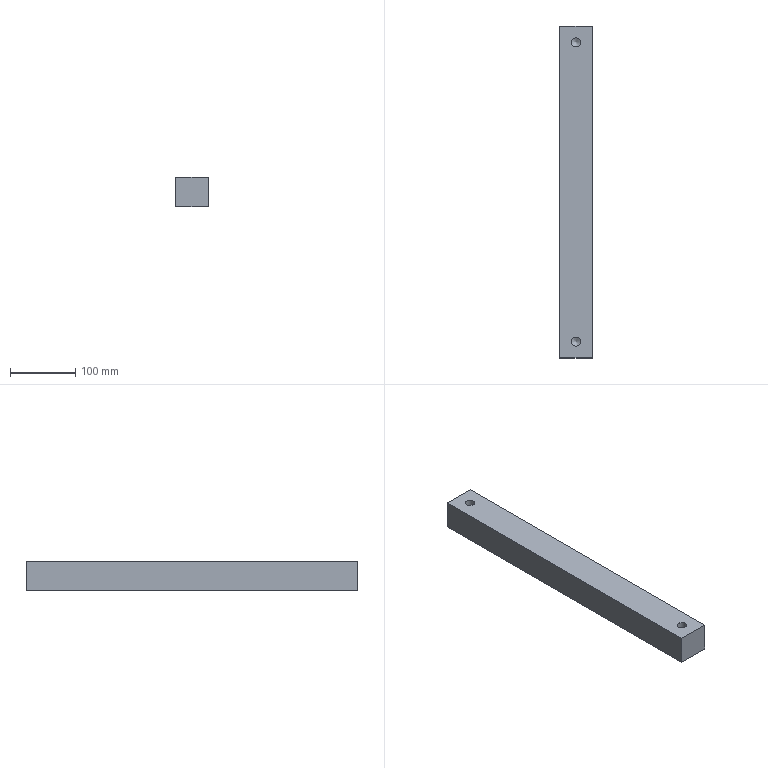Part | STEP file | 023_id2182_x_t | 1 solid | 10 faces | box 50 x 510 x 45 mm | volume 1141094 mm3 | plane 6 | cylinder 2 | cone 2 | commonest cylinder face diameters 14 x2
STEP:
#1=CARTESIAN_POINT('',(0.,0.,0.));
#2=DIRECTION('',(0.,0.,1.));
#3=DIRECTION('',(1.,0.,0.));
#4=AXIS2_PLACEMENT_3D('',#1,#2,#3);
#5=CARTESIAN_POINT('',(716.5,230.,230.));
#6=VERTEX_POINT('',#5);
#7=CARTESIAN_POINT('',(730.5,230.,230.));
#8=VERTEX_POINT('',#7);
#9=CARTESIAN_POINT('',(723.5,230.,230.));
#10=DIRECTION('',(0.,0.,1.));
#11=DIRECTION('',(-1.,0.,0.));
#12=AXIS2_PLACEMENT_3D('',#9,#10,#11);
#13=CIRCLE('',#12,7.);
#14=CARTESIAN_POINT('',(903.5,-140.,230.));
#15=DIRECTION('',(0.,0.,1.));
#16=DIRECTION('',(1.,0.,0.));
#17=AXIS2_PLACEMENT_3D('',#14,#15,#16);
#18=PLANE('',#17);
#19=CARTESIAN_POINT('',(-180.,370.));
#20=DIRECTION('',(-1.,0.));
#21=AXIS2_PLACEMENT_2D('',#19,#20);
#22=CIRCLE('',#21,7.);
#23=(GEOMETRIC_REPRESENTATION_CONTEXT(2)PARAMETRIC_REPRESENTATION_CONTEXT()REPRESENTATION_CONTEXT('',''));
#24=DEFINITIONAL_REPRESENTATION('',(#22),#23);
#25=PCURVE('',#18,#24);
#26=CARTESIAN_POINT('',(723.5,230.,279.));
#27=DIRECTION('',(0.,0.,-1.));
#28=DIRECTION('',(1.,0.,0.));
#29=AXIS2_PLACEMENT_3D('',#26,#27,#28);
#30=CYLINDRICAL_SURFACE('',#29,7.);
#31=CARTESIAN_POINT('',(3.142,49.));
#32=DIRECTION('',(-1.,0.));
#33=VECTOR('',#32,1.);
#34=LINE('',#31,#33);
#35=(GEOMETRIC_REPRESENTATION_CONTEXT(2)PARAMETRIC_REPRESENTATION_CONTEXT()REPRESENTATION_CONTEXT('',''));
#36=DEFINITIONAL_REPRESENTATION('',(#34),#35);
#37=PCURVE('',#30,#36);
#38=SURFACE_CURVE('',#13,(#25,#37),.PCURVE_S1.);
#39=EDGE_CURVE('',#6,#8,#38,.T.);
#40=ORIENTED_EDGE('',*,*,#39,.F.);
#41=CARTESIAN_POINT('',(723.5,230.,230.));
#42=DIRECTION('',(0.,0.,1.));
#43=DIRECTION('',(-1.,0.,0.));
#44=AXIS2_PLACEMENT_3D('',#41,#42,#43);
#45=CIRCLE('',#44,7.);
#46=CARTESIAN_POINT('',(-180.,370.));
#47=DIRECTION('',(-1.,0.));
#48=AXIS2_PLACEMENT_2D('',#46,#47);
#49=CIRCLE('',#48,7.);
#50=(GEOMETRIC_REPRESENTATION_CONTEXT(2)PARAMETRIC_REPRESENTATION_CONTEXT()REPRESENTATION_CONTEXT('',''));
#51=DEFINITIONAL_REPRESENTATION('',(#49),#50);
#52=PCURVE('',#18,#51);
#53=CARTESIAN_POINT('',(9.425,49.));
#54=DIRECTION('',(-1.,0.));
#55=VECTOR('',#54,1.);
#56=LINE('',#53,#55);
#57=(GEOMETRIC_REPRESENTATION_CONTEXT(2)PARAMETRIC_REPRESENTATION_CONTEXT()REPRESENTATION_CONTEXT('',''));
#58=DEFINITIONAL_REPRESENTATION('',(#56),#57);
#59=PCURVE('',#30,#58);
#60=SURFACE_CURVE('',#45,(#52,#59),.PCURVE_S1.);
#61=EDGE_CURVE('',#8,#6,#60,.T.);
#62=ORIENTED_EDGE('',*,*,#61,.F.);
#63=EDGE_LOOP('',(#40,#62));
#64=FACE_BOUND('',#63,.T.);
#65=CARTESIAN_POINT('',(716.5,-230.,230.));
#66=VERTEX_POINT('',#65);
#67=CARTESIAN_POINT('',(730.5,-230.,230.));
#68=VERTEX_POINT('',#67);
#69=CARTESIAN_POINT('',(723.5,-230.,230.));
#70=DIRECTION('',(0.,0.,-1.));
#71=DIRECTION('',(-1.,0.,0.));
#72=AXIS2_PLACEMENT_3D('',#69,#70,#71);
#73=CIRCLE('',#72,7.);
#74=CARTESIAN_POINT('',(-187.,-90.));
#75=CARTESIAN_POINT('',(-187.,-77.876));
#76=CARTESIAN_POINT('',(-176.5,-83.938));
#77=CARTESIAN_POINT('',(-166.,-90.));
#78=CARTESIAN_POINT('',(-176.5,-96.062));
#79=CARTESIAN_POINT('',(-187.,-102.124));
#80=CARTESIAN_POINT('',(-187.,-90.));
#81=(BOUNDED_CURVE()B_SPLINE_CURVE(2,(#74,#75,#76,#77,#78,#79,#80),.UNSPECIFIED.,.T.,.F.)B_SPLINE_CURVE_WITH_KNOTS((1,2,2,2,2,1),(-2.094,0.,2.094,4.189,6.283,8.378),.UNSPECIFIED.)CURVE()GEOMETRIC_REPRESENTATION_ITEM()RATIONAL_B_SPLINE_CURVE((1.,0.5,1.,0.5,1.,0.5,1.))REPRESENTATION_ITEM(''));
#82=(GEOMETRIC_REPRESENTATION_CONTEXT(2)PARAMETRIC_REPRESENTATION_CONTEXT()REPRESENTATION_CONTEXT('',''));
#83=DEFINITIONAL_REPRESENTATION('',(#81),#82);
#84=PCURVE('',#18,#83);
#85=CARTESIAN_POINT('',(723.5,-230.,279.));
#86=DIRECTION('',(0.,0.,-1.));
#87=DIRECTION('',(1.,0.,0.));
#88=AXIS2_PLACEMENT_3D('',#85,#86,#87);
#89=CYLINDRICAL_SURFACE('',#88,7.);
#90=CARTESIAN_POINT('',(3.142,49.));
#91=DIRECTION('',(1.,0.));
#92=VECTOR('',#91,1.);
#93=LINE('',#90,#92);
#94=(GEOMETRIC_REPRESENTATION_CONTEXT(2)PARAMETRIC_REPRESENTATION_CONTEXT()REPRESENTATION_CONTEXT('',''));
#95=DEFINITIONAL_REPRESENTATION('',(#93),#94);
#96=PCURVE('',#89,#95);
#97=SURFACE_CURVE('',#73,(#84,#96),.PCURVE_S1.);
#98=EDGE_CURVE('',#66,#68,#97,.T.);
#99=ORIENTED_EDGE('',*,*,#98,.T.);
#100=CARTESIAN_POINT('',(723.5,-230.,230.));
#101=DIRECTION('',(0.,0.,-1.));
#102=DIRECTION('',(-1.,0.,0.));
#103=AXIS2_PLACEMENT_3D('',#100,#101,#102);
#104=CIRCLE('',#103,7.);
#105=CARTESIAN_POINT('',(-187.,-90.));
#106=CARTESIAN_POINT('',(-187.,-77.876));
#107=CARTESIAN_POINT('',(-176.5,-83.938));
#108=CARTESIAN_POINT('',(-166.,-90.));
#109=CARTESIAN_POINT('',(-176.5,-96.062));
#110=CARTESIAN_POINT('',(-187.,-102.124));
#111=CARTESIAN_POINT('',(-187.,-90.));
#112=(BOUNDED_CURVE()B_SPLINE_CURVE(2,(#105,#106,#107,#108,#109,#110,#111),.UNSPECIFIED.,.T.,.F.)B_SPLINE_CURVE_WITH_KNOTS((1,2,2,2,2,1),(-2.094,0.,2.094,4.189,6.283,8.378),.UNSPECIFIED.)CURVE()GEOMETRIC_REPRESENTATION_ITEM()RATIONAL_B_SPLINE_CURVE((1.,0.5,1.,0.5,1.,0.5,1.))REPRESENTATION_ITEM(''));
#113=(GEOMETRIC_REPRESENTATION_CONTEXT(2)PARAMETRIC_REPRESENTATION_CONTEXT()REPRESENTATION_CONTEXT('',''));
#114=DEFINITIONAL_REPRESENTATION('',(#112),#113);
#115=PCURVE('',#18,#114);
#116=CARTESIAN_POINT('',(-3.142,49.));
#117=DIRECTION('',(1.,0.));
#118=VECTOR('',#117,1.);
#119=LINE('',#116,#118);
#120=(GEOMETRIC_REPRESENTATION_CONTEXT(2)PARAMETRIC_REPRESENTATION_CONTEXT()REPRESENTATION_CONTEXT('',''));
#121=DEFINITIONAL_REPRESENTATION('',(#119),#120);
#122=PCURVE('',#89,#121);
#123=SURFACE_CURVE('',#104,(#115,#122),.PCURVE_S1.);
#124=EDGE_CURVE('',#68,#66,#123,.T.);
#125=ORIENTED_EDGE('',*,*,#124,.T.);
#126=EDGE_LOOP('',(#99,#125));
#127=FACE_BOUND('',#126,.T.);
#128=CARTESIAN_POINT('',(748.5,255.,230.));
#129=VERTEX_POINT('',#128);
#130=CARTESIAN_POINT('',(698.5,255.,230.));
#131=VERTEX_POINT('',#130);
#132=CARTESIAN_POINT('',(698.5,255.,230.));
#133=DIRECTION('',(-1.,0.,0.));
#134=VECTOR('',#133,1.);
#135=LINE('',#132,#134);
#136=CARTESIAN_POINT('',(-205.,395.));
#137=DIRECTION('',(-1.,0.));
#138=VECTOR('',#137,1.);
#139=LINE('',#136,#138);
#140=(GEOMETRIC_REPRESENTATION_CONTEXT(2)PARAMETRIC_REPRESENTATION_CONTEXT()REPRESENTATION_CONTEXT('',''));
#141=DEFINITIONAL_REPRESENTATION('',(#139),#140);
#142=PCURVE('',#18,#141);
#143=CARTESIAN_POINT('',(698.5,255.,428.5));
#144=DIRECTION('',(0.,1.,0.));
#145=DIRECTION('',(0.,0.,1.));
#146=AXIS2_PLACEMENT_3D('',#143,#144,#145);
#147=PLANE('',#146);
#148=CARTESIAN_POINT('',(-198.5,0.));
#149=DIRECTION('',(0.,-1.));
#150=VECTOR('',#149,1.);
#151=LINE('',#148,#150);
#152=(GEOMETRIC_REPRESENTATION_CONTEXT(2)PARAMETRIC_REPRESENTATION_CONTEXT()REPRESENTATION_CONTEXT('',''));
#153=DEFINITIONAL_REPRESENTATION('',(#151),#152);
#154=PCURVE('',#147,#153);
#155=SURFACE_CURVE('',#135,(#142,#154),.PCURVE_S1.);
#156=EDGE_CURVE('',#129,#131,#155,.T.);
#157=ORIENTED_EDGE('',*,*,#156,.T.);
#158=CARTESIAN_POINT('',(698.5,-255.,230.));
#159=VERTEX_POINT('',#158);
#160=CARTESIAN_POINT('',(698.5,-350.,230.));
#161=DIRECTION('',(0.,-1.,0.));
#162=VECTOR('',#161,1.);
#163=LINE('',#160,#162);
#164=CARTESIAN_POINT('',(-205.,-210.));
#165=DIRECTION('',(0.,-1.));
#166=VECTOR('',#165,1.);
#167=LINE('',#164,#166);
#168=(GEOMETRIC_REPRESENTATION_CONTEXT(2)PARAMETRIC_REPRESENTATION_CONTEXT()REPRESENTATION_CONTEXT('',''));
#169=DEFINITIONAL_REPRESENTATION('',(#167),#168);
#170=PCURVE('',#18,#169);
#171=CARTESIAN_POINT('',(698.5,-350.,428.5));
#172=DIRECTION('',(-1.,0.,0.));
#173=DIRECTION('',(0.,0.,-1.));
#174=AXIS2_PLACEMENT_3D('',#171,#172,#173);
#175=PLANE('',#174);
#176=CARTESIAN_POINT('',(198.5,0.));
#177=DIRECTION('',(0.,1.));
#178=VECTOR('',#177,1.);
#179=LINE('',#176,#178);
#180=(GEOMETRIC_REPRESENTATION_CONTEXT(2)PARAMETRIC_REPRESENTATION_CONTEXT()REPRESENTATION_CONTEXT('',''));
#181=DEFINITIONAL_REPRESENTATION('',(#179),#180);
#182=PCURVE('',#175,#181);
#183=SURFACE_CURVE('',#163,(#170,#182),.PCURVE_S1.);
#184=EDGE_CURVE('',#131,#159,#183,.T.);
#185=ORIENTED_EDGE('',*,*,#184,.T.);
#186=CARTESIAN_POINT('',(748.5,-255.,230.));
#187=VERTEX_POINT('',#186);
#188=CARTESIAN_POINT('',(698.5,-255.,230.));
#189=DIRECTION('',(-1.,0.,0.));
#190=VECTOR('',#189,1.);
#191=LINE('',#188,#190);
#192=CARTESIAN_POINT('',(-205.,-115.));
#193=DIRECTION('',(-1.,0.));
#194=VECTOR('',#193,1.);
#195=LINE('',#192,#194);
#196=(GEOMETRIC_REPRESENTATION_CONTEXT(2)PARAMETRIC_REPRESENTATION_CONTEXT()REPRESENTATION_CONTEXT('',''));
#197=DEFINITIONAL_REPRESENTATION('',(#195),#196);
#198=PCURVE('',#18,#197);
#199=CARTESIAN_POINT('',(698.5,-255.,428.5));
#200=DIRECTION('',(0.,1.,0.));
#201=DIRECTION('',(0.,0.,1.));
#202=AXIS2_PLACEMENT_3D('',#199,#200,#201);
#203=PLANE('',#202);
#204=CARTESIAN_POINT('',(-198.5,0.));
#205=DIRECTION('',(0.,-1.));
#206=VECTOR('',#205,1.);
#207=LINE('',#204,#206);
#208=(GEOMETRIC_REPRESENTATION_CONTEXT(2)PARAMETRIC_REPRESENTATION_CONTEXT()REPRESENTATION_CONTEXT('',''));
#209=DEFINITIONAL_REPRESENTATION('',(#207),#208);
#210=PCURVE('',#203,#209);
#211=SURFACE_CURVE('',#191,(#198,#210),.PCURVE_S1.);
#212=EDGE_CURVE('',#187,#159,#211,.T.);
#213=ORIENTED_EDGE('',*,*,#212,.F.);
#214=CARTESIAN_POINT('',(748.5,-350.,230.));
#215=DIRECTION('',(0.,1.,0.));
#216=VECTOR('',#215,1.);
#217=LINE('',#214,#216);
#218=CARTESIAN_POINT('',(-155.,-210.));
#219=DIRECTION('',(0.,1.));
#220=VECTOR('',#219,1.);
#221=LINE('',#218,#220);
#222=(GEOMETRIC_REPRESENTATION_CONTEXT(2)PARAMETRIC_REPRESENTATION_CONTEXT()REPRESENTATION_CONTEXT('',''));
#223=DEFINITIONAL_REPRESENTATION('',(#221),#222);
#224=PCURVE('',#18,#223);
#225=CARTESIAN_POINT('',(748.5,-350.,428.5));
#226=DIRECTION('',(-1.,0.,0.));
#227=DIRECTION('',(0.,0.,-1.));
#228=AXIS2_PLACEMENT_3D('',#225,#226,#227);
#229=PLANE('',#228);
#230=CARTESIAN_POINT('',(198.5,0.));
#231=DIRECTION('',(0.,-1.));
#232=VECTOR('',#231,1.);
#233=LINE('',#230,#232);
#234=(GEOMETRIC_REPRESENTATION_CONTEXT(2)PARAMETRIC_REPRESENTATION_CONTEXT()REPRESENTATION_CONTEXT('',''));
#235=DEFINITIONAL_REPRESENTATION('',(#233),#234);
#236=PCURVE('',#229,#235);
#237=SURFACE_CURVE('',#217,(#224,#236),.PCURVE_S1.);
#238=EDGE_CURVE('',#187,#129,#237,.T.);
#239=ORIENTED_EDGE('',*,*,#238,.T.);
#240=EDGE_LOOP('',(#157,#185,#213,#239));
#241=FACE_BOUND('',#240,.T.);
#242=ADVANCED_FACE('',(#64,#127,#241),#18,.T.);
#243=CARTESIAN_POINT('',(748.5,-255.,185.));
#244=VERTEX_POINT('',#243);
#245=CARTESIAN_POINT('',(698.5,-255.,185.));
#246=VERTEX_POINT('',#245);
#247=CARTESIAN_POINT('',(698.5,-255.,185.));
#248=DIRECTION('',(-1.,0.,0.));
#249=VECTOR('',#248,1.);
#250=LINE('',#247,#249);
#251=CARTESIAN_POINT('',(698.5,-350.,185.));
#252=DIRECTION('',(0.,0.,1.));
#253=DIRECTION('',(0.,-1.,0.));
#254=AXIS2_PLACEMENT_3D('',#251,#252,#253);
#255=PLANE('',#254);
#256=CARTESIAN_POINT('',(-95.,0.));
#257=DIRECTION('',(0.,-1.));
#258=VECTOR('',#257,1.);
#259=LINE('',#256,#258);
#260=(GEOMETRIC_REPRESENTATION_CONTEXT(2)PARAMETRIC_REPRESENTATION_CONTEXT()REPRESENTATION_CONTEXT('',''));
#261=DEFINITIONAL_REPRESENTATION('',(#259),#260);
#262=PCURVE('',#255,#261);
#263=CARTESIAN_POINT('',(-243.5,0.));
#264=DIRECTION('',(0.,-1.));
#265=VECTOR('',#264,1.);
#266=LINE('',#263,#265);
#267=(GEOMETRIC_REPRESENTATION_CONTEXT(2)PARAMETRIC_REPRESENTATION_CONTEXT()REPRESENTATION_CONTEXT('',''));
#268=DEFINITIONAL_REPRESENTATION('',(#266),#267);
#269=PCURVE('',#203,#268);
#270=SURFACE_CURVE('',#250,(#262,#269),.PCURVE_S1.);
#271=EDGE_CURVE('',#244,#246,#270,.T.);
#272=ORIENTED_EDGE('',*,*,#271,.T.);
#273=CARTESIAN_POINT('',(698.5,255.,185.));
#274=VERTEX_POINT('',#273);
#275=CARTESIAN_POINT('',(698.5,-350.,185.));
#276=DIRECTION('',(0.,1.,0.));
#277=VECTOR('',#276,1.);
#278=LINE('',#275,#277);
#279=CARTESIAN_POINT('',(0.,0.));
#280=DIRECTION('',(-1.,0.));
#281=VECTOR('',#280,1.);
#282=LINE('',#279,#281);
#283=(GEOMETRIC_REPRESENTATION_CONTEXT(2)PARAMETRIC_REPRESENTATION_CONTEXT()REPRESENTATION_CONTEXT('',''));
#284=DEFINITIONAL_REPRESENTATION('',(#282),#283);
#285=PCURVE('',#255,#284);
#286=CARTESIAN_POINT('',(243.5,0.));
#287=DIRECTION('',(0.,-1.));
#288=VECTOR('',#287,1.);
#289=LINE('',#286,#288);
#290=(GEOMETRIC_REPRESENTATION_CONTEXT(2)PARAMETRIC_REPRESENTATION_CONTEXT()REPRESENTATION_CONTEXT('',''));
#291=DEFINITIONAL_REPRESENTATION('',(#289),#290);
#292=PCURVE('',#175,#291);
#293=SURFACE_CURVE('',#278,(#285,#292),.PCURVE_S1.);
#294=EDGE_CURVE('',#246,#274,#293,.T.);
#295=ORIENTED_EDGE('',*,*,#294,.T.);
#296=CARTESIAN_POINT('',(748.5,255.,185.));
#297=VERTEX_POINT('',#296);
#298=CARTESIAN_POINT('',(698.5,255.,185.));
#299=DIRECTION('',(-1.,0.,0.));
#300=VECTOR('',#299,1.);
#301=LINE('',#298,#300);
#302=CARTESIAN_POINT('',(-605.,0.));
#303=DIRECTION('',(0.,-1.));
#304=VECTOR('',#303,1.);
#305=LINE('',#302,#304);
#306=(GEOMETRIC_REPRESENTATION_CONTEXT(2)PARAMETRIC_REPRESENTATION_CONTEXT()REPRESENTATION_CONTEXT('',''));
#307=DEFINITIONAL_REPRESENTATION('',(#305),#306);
#308=PCURVE('',#255,#307);
#309=CARTESIAN_POINT('',(-243.5,0.));
#310=DIRECTION('',(0.,-1.));
#311=VECTOR('',#310,1.);
#312=LINE('',#309,#311);
#313=(GEOMETRIC_REPRESENTATION_CONTEXT(2)PARAMETRIC_REPRESENTATION_CONTEXT()REPRESENTATION_CONTEXT('',''));
#314=DEFINITIONAL_REPRESENTATION('',(#312),#313);
#315=PCURVE('',#147,#314);
#316=SURFACE_CURVE('',#301,(#308,#315),.PCURVE_S1.);
#317=EDGE_CURVE('',#297,#274,#316,.T.);
#318=ORIENTED_EDGE('',*,*,#317,.F.);
#319=CARTESIAN_POINT('',(748.5,-350.,185.));
#320=DIRECTION('',(0.,1.,0.));
#321=VECTOR('',#320,1.);
#322=LINE('',#319,#321);
#323=CARTESIAN_POINT('',(0.,50.));
#324=DIRECTION('',(-1.,0.));
#325=VECTOR('',#324,1.);
#326=LINE('',#323,#325);
#327=(GEOMETRIC_REPRESENTATION_CONTEXT(2)PARAMETRIC_REPRESENTATION_CONTEXT()REPRESENTATION_CONTEXT('',''));
#328=DEFINITIONAL_REPRESENTATION('',(#326),#327);
#329=PCURVE('',#255,#328);
#330=CARTESIAN_POINT('',(243.5,0.));
#331=DIRECTION('',(0.,-1.));
#332=VECTOR('',#331,1.);
#333=LINE('',#330,#332);
#334=(GEOMETRIC_REPRESENTATION_CONTEXT(2)PARAMETRIC_REPRESENTATION_CONTEXT()REPRESENTATION_CONTEXT('',''));
#335=DEFINITIONAL_REPRESENTATION('',(#333),#334);
#336=PCURVE('',#229,#335);
#337=SURFACE_CURVE('',#322,(#329,#336),.PCURVE_S1.);
#338=EDGE_CURVE('',#244,#297,#337,.T.);
#339=ORIENTED_EDGE('',*,*,#338,.F.);
#340=EDGE_LOOP('',(#272,#295,#318,#339));
#341=FACE_BOUND('',#340,.T.);
#342=ADVANCED_FACE('',(#341),#255,.F.);
#343=ORIENTED_EDGE('',*,*,#238,.F.);
#344=CARTESIAN_POINT('',(748.5,-255.,428.5));
#345=DIRECTION('',(0.,0.,-1.));
#346=VECTOR('',#345,1.);
#347=LINE('',#344,#346);
#348=CARTESIAN_POINT('',(0.,-95.));
#349=DIRECTION('',(1.,0.));
#350=VECTOR('',#349,1.);
#351=LINE('',#348,#350);
#352=(GEOMETRIC_REPRESENTATION_CONTEXT(2)PARAMETRIC_REPRESENTATION_CONTEXT()REPRESENTATION_CONTEXT('',''));
#353=DEFINITIONAL_REPRESENTATION('',(#351),#352);
#354=PCURVE('',#229,#353);
#355=CARTESIAN_POINT('',(0.,50.));
#356=DIRECTION('',(-1.,0.));
#357=VECTOR('',#356,1.);
#358=LINE('',#355,#357);
#359=(GEOMETRIC_REPRESENTATION_CONTEXT(2)PARAMETRIC_REPRESENTATION_CONTEXT()REPRESENTATION_CONTEXT('',''));
#360=DEFINITIONAL_REPRESENTATION('',(#358),#359);
#361=PCURVE('',#203,#360);
#362=SURFACE_CURVE('',#347,(#354,#361),.PCURVE_S1.);
#363=EDGE_CURVE('',#187,#244,#362,.T.);
#364=ORIENTED_EDGE('',*,*,#363,.T.);
#365=ORIENTED_EDGE('',*,*,#338,.T.);
#366=CARTESIAN_POINT('',(748.5,255.,428.5));
#367=DIRECTION('',(0.,0.,1.));
#368=VECTOR('',#367,1.);
#369=LINE('',#366,#368);
#370=CARTESIAN_POINT('',(0.,-605.));
#371=DIRECTION('',(-1.,0.));
#372=VECTOR('',#371,1.);
#373=LINE('',#370,#372);
#374=(GEOMETRIC_REPRESENTATION_CONTEXT(2)PARAMETRIC_REPRESENTATION_CONTEXT()REPRESENTATION_CONTEXT('',''));
#375=DEFINITIONAL_REPRESENTATION('',(#373),#374);
#376=PCURVE('',#229,#375);
#377=CARTESIAN_POINT('',(0.,50.));
#378=DIRECTION('',(1.,0.));
#379=VECTOR('',#378,1.);
#380=LINE('',#377,#379);
#381=(GEOMETRIC_REPRESENTATION_CONTEXT(2)PARAMETRIC_REPRESENTATION_CONTEXT()REPRESENTATION_CONTEXT('',''));
#382=DEFINITIONAL_REPRESENTATION('',(#380),#381);
#383=PCURVE('',#147,#382);
#384=SURFACE_CURVE('',#369,(#376,#383),.PCURVE_S1.);
#385=EDGE_CURVE('',#297,#129,#384,.T.);
#386=ORIENTED_EDGE('',*,*,#385,.T.);
#387=EDGE_LOOP('',(#343,#364,#365,#386));
#388=FACE_BOUND('',#387,.T.);
#389=ADVANCED_FACE('',(#388),#229,.F.);
#390=ORIENTED_EDGE('',*,*,#212,.T.);
#391=CARTESIAN_POINT('',(698.5,-255.,428.5));
#392=DIRECTION('',(0.,0.,-1.));
#393=VECTOR('',#392,1.);
#394=LINE('',#391,#393);
#395=CARTESIAN_POINT('',(0.,0.));
#396=DIRECTION('',(-1.,0.));
#397=VECTOR('',#396,1.);
#398=LINE('',#395,#397);
#399=(GEOMETRIC_REPRESENTATION_CONTEXT(2)PARAMETRIC_REPRESENTATION_CONTEXT()REPRESENTATION_CONTEXT('',''));
#400=DEFINITIONAL_REPRESENTATION('',(#398),#399);
#401=PCURVE('',#203,#400);
#402=CARTESIAN_POINT('',(0.,-95.));
#403=DIRECTION('',(1.,0.));
#404=VECTOR('',#403,1.);
#405=LINE('',#402,#404);
#406=(GEOMETRIC_REPRESENTATION_CONTEXT(2)PARAMETRIC_REPRESENTATION_CONTEXT()REPRESENTATION_CONTEXT('',''));
#407=DEFINITIONAL_REPRESENTATION('',(#405),#406);
#408=PCURVE('',#175,#407);
#409=SURFACE_CURVE('',#394,(#401,#408),.PCURVE_S1.);
#410=EDGE_CURVE('',#159,#246,#409,.T.);
#411=ORIENTED_EDGE('',*,*,#410,.T.);
#412=ORIENTED_EDGE('',*,*,#271,.F.);
#413=ORIENTED_EDGE('',*,*,#363,.F.);
#414=EDGE_LOOP('',(#390,#411,#412,#413));
#415=FACE_BOUND('',#414,.T.);
#416=ADVANCED_FACE('',(#415),#203,.F.);
#417=CARTESIAN_POINT('',(698.5,255.,428.5));
#418=DIRECTION('',(0.,0.,1.));
#419=VECTOR('',#418,1.);
#420=LINE('',#417,#419);
#421=CARTESIAN_POINT('',(0.,-605.));
#422=DIRECTION('',(-1.,0.));
#423=VECTOR('',#422,1.);
#424=LINE('',#421,#423);
#425=(GEOMETRIC_REPRESENTATION_CONTEXT(2)PARAMETRIC_REPRESENTATION_CONTEXT()REPRESENTATION_CONTEXT('',''));
#426=DEFINITIONAL_REPRESENTATION('',(#424),#425);
#427=PCURVE('',#175,#426);
#428=CARTESIAN_POINT('',(0.,0.));
#429=DIRECTION('',(1.,0.));
#430=VECTOR('',#429,1.);
#431=LINE('',#428,#430);
#432=(GEOMETRIC_REPRESENTATION_CONTEXT(2)PARAMETRIC_REPRESENTATION_CONTEXT()REPRESENTATION_CONTEXT('',''));
#433=DEFINITIONAL_REPRESENTATION('',(#431),#432);
#434=PCURVE('',#147,#433);
#435=SURFACE_CURVE('',#420,(#427,#434),.PCURVE_S1.);
#436=EDGE_CURVE('',#274,#131,#435,.T.);
#437=ORIENTED_EDGE('',*,*,#436,.F.);
#438=ORIENTED_EDGE('',*,*,#294,.F.);
#439=ORIENTED_EDGE('',*,*,#410,.F.);
#440=ORIENTED_EDGE('',*,*,#184,.F.);
#441=EDGE_LOOP('',(#437,#438,#439,#440));
#442=FACE_BOUND('',#441,.T.);
#443=ADVANCED_FACE('',(#442),#175,.T.);
#444=ORIENTED_EDGE('',*,*,#385,.F.);
#445=ORIENTED_EDGE('',*,*,#317,.T.);
#446=ORIENTED_EDGE('',*,*,#436,.T.);
#447=ORIENTED_EDGE('',*,*,#156,.F.);
#448=EDGE_LOOP('',(#444,#445,#446,#447));
#449=FACE_BOUND('',#448,.T.);
#450=ADVANCED_FACE('',(#449),#147,.T.);
#451=ORIENTED_EDGE('',*,*,#61,.F.);
#452=CARTESIAN_POINT('',(730.5,230.,210.541));
#453=VERTEX_POINT('',#452);
#454=CARTESIAN_POINT('',(730.5,230.,230.));
#455=CARTESIAN_POINT('',(730.5,230.,210.541));
#456=B_SPLINE_CURVE_WITH_KNOTS('',1,(#454,#455),.UNSPECIFIED.,.F.,.F.,(2,2),(49.,68.459),.PIECEWISE_BEZIER_KNOTS.);
#457=CARTESIAN_POINT('',(6.283,0.));
#458=DIRECTION('',(0.,1.));
#459=VECTOR('',#458,1.);
#460=LINE('',#457,#459);
#461=(GEOMETRIC_REPRESENTATION_CONTEXT(2)PARAMETRIC_REPRESENTATION_CONTEXT()REPRESENTATION_CONTEXT('',''));
#462=DEFINITIONAL_REPRESENTATION('',(#460),#461);
#463=PCURVE('',#30,#462);
#464=CARTESIAN_POINT('',(0.,0.));
#465=DIRECTION('',(0.,1.));
#466=VECTOR('',#465,1.);
#467=LINE('',#464,#466);
#468=(GEOMETRIC_REPRESENTATION_CONTEXT(2)PARAMETRIC_REPRESENTATION_CONTEXT()REPRESENTATION_CONTEXT('',''));
#469=DEFINITIONAL_REPRESENTATION('',(#467),#468);
#470=PCURVE('',#30,#469);
#471=SEAM_CURVE('',#456,(#463,#470),.PCURVE_S1.);
#472=EDGE_CURVE('',#8,#453,#471,.T.);
#473=ORIENTED_EDGE('',*,*,#472,.T.);
#474=CARTESIAN_POINT('',(716.5,230.,210.541));
#475=VERTEX_POINT('',#474);
#476=CARTESIAN_POINT('',(723.5,230.,210.541));
#477=DIRECTION('',(0.,0.,1.));
#478=DIRECTION('',(1.,0.,0.));
#479=AXIS2_PLACEMENT_3D('',#476,#477,#478);
#480=CIRCLE('',#479,7.);
#481=CARTESIAN_POINT('',(6.283,68.459));
#482=DIRECTION('',(-1.,0.));
#483=VECTOR('',#482,1.);
#484=LINE('',#481,#483);
#485=(GEOMETRIC_REPRESENTATION_CONTEXT(2)PARAMETRIC_REPRESENTATION_CONTEXT()REPRESENTATION_CONTEXT('',''));
#486=DEFINITIONAL_REPRESENTATION('',(#484),#485);
#487=PCURVE('',#30,#486);
#488=CARTESIAN_POINT('',(723.5,230.,210.541));
#489=DIRECTION('',(0.,0.,1.));
#490=DIRECTION('',(-1.,0.,0.));
#491=AXIS2_PLACEMENT_3D('',#488,#489,#490);
#492=CONICAL_SURFACE('',#491,7.,1.047);
#493=CARTESIAN_POINT('',(3.142,0.));
#494=DIRECTION('',(1.,0.));
#495=VECTOR('',#494,1.);
#496=LINE('',#493,#495);
#497=(GEOMETRIC_REPRESENTATION_CONTEXT(2)PARAMETRIC_REPRESENTATION_CONTEXT()REPRESENTATION_CONTEXT('',''));
#498=DEFINITIONAL_REPRESENTATION('',(#496),#497);
#499=PCURVE('',#492,#498);
#500=SURFACE_CURVE('',#480,(#487,#499),.PCURVE_S1.);
#501=EDGE_CURVE('',#453,#475,#500,.T.);
#502=ORIENTED_EDGE('',*,*,#501,.T.);
#503=CARTESIAN_POINT('',(723.5,230.,210.541));
#504=DIRECTION('',(0.,0.,1.));
#505=DIRECTION('',(1.,0.,0.));
#506=AXIS2_PLACEMENT_3D('',#503,#504,#505);
#507=CIRCLE('',#506,7.);
#508=CARTESIAN_POINT('',(6.283,68.459));
#509=DIRECTION('',(-1.,0.));
#510=VECTOR('',#509,1.);
#511=LINE('',#508,#510);
#512=(GEOMETRIC_REPRESENTATION_CONTEXT(2)PARAMETRIC_REPRESENTATION_CONTEXT()REPRESENTATION_CONTEXT('',''));
#513=DEFINITIONAL_REPRESENTATION('',(#511),#512);
#514=PCURVE('',#30,#513);
#515=CARTESIAN_POINT('',(-3.142,0.));
#516=DIRECTION('',(1.,0.));
#517=VECTOR('',#516,1.);
#518=LINE('',#515,#517);
#519=(GEOMETRIC_REPRESENTATION_CONTEXT(2)PARAMETRIC_REPRESENTATION_CONTEXT()REPRESENTATION_CONTEXT('',''));
#520=DEFINITIONAL_REPRESENTATION('',(#518),#519);
#521=PCURVE('',#492,#520);
#522=SURFACE_CURVE('',#507,(#514,#521),.PCURVE_S1.);
#523=EDGE_CURVE('',#475,#453,#522,.T.);
#524=ORIENTED_EDGE('',*,*,#523,.T.);
#525=ORIENTED_EDGE('',*,*,#472,.F.);
#526=ORIENTED_EDGE('',*,*,#39,.F.);
#527=EDGE_LOOP('',(#451,#473,#502,#524,#525,#526));
#528=FACE_BOUND('',#527,.F.);
#529=ADVANCED_FACE('',(#528),#30,.F.);
#530=CARTESIAN_POINT('',(723.5,230.,206.5));
#531=VERTEX_POINT('',#530);
#532=CARTESIAN_POINT('',(723.5,230.,206.5));
#533=CARTESIAN_POINT('',(716.5,230.,210.541));
#534=B_SPLINE_CURVE_WITH_KNOTS('',1,(#532,#533),.UNSPECIFIED.,.F.,.F.,(2,2),(-8.083,0.),.PIECEWISE_BEZIER_KNOTS.);
#535=CARTESIAN_POINT('',(6.283,0.));
#536=DIRECTION('',(0.,1.));
#537=VECTOR('',#536,1.);
#538=LINE('',#535,#537);
#539=(GEOMETRIC_REPRESENTATION_CONTEXT(2)PARAMETRIC_REPRESENTATION_CONTEXT()REPRESENTATION_CONTEXT('',''));
#540=DEFINITIONAL_REPRESENTATION('',(#538),#539);
#541=PCURVE('',#492,#540);
#542=CARTESIAN_POINT('',(0.,0.));
#543=DIRECTION('',(0.,1.));
#544=VECTOR('',#543,1.);
#545=LINE('',#542,#544);
#546=(GEOMETRIC_REPRESENTATION_CONTEXT(2)PARAMETRIC_REPRESENTATION_CONTEXT()REPRESENTATION_CONTEXT('',''));
#547=DEFINITIONAL_REPRESENTATION('',(#545),#546);
#548=PCURVE('',#492,#547);
#549=SEAM_CURVE('',#534,(#541,#548),.PCURVE_S1.);
#550=EDGE_CURVE('',#531,#475,#549,.T.);
#551=ORIENTED_EDGE('',*,*,#550,.T.);
#552=ORIENTED_EDGE('',*,*,#501,.F.);
#553=ORIENTED_EDGE('',*,*,#523,.F.);
#554=ORIENTED_EDGE('',*,*,#550,.F.);
#555=EDGE_LOOP('',(#551,#552,#553,#554));
#556=FACE_BOUND('',#555,.F.);
#557=ADVANCED_FACE('',(#556),#492,.F.);
#558=ORIENTED_EDGE('',*,*,#98,.T.);
#559=CARTESIAN_POINT('',(730.5,-230.,210.541));
#560=VERTEX_POINT('',#559);
#561=CARTESIAN_POINT('',(730.5,-230.,230.));
#562=CARTESIAN_POINT('',(730.5,-230.,210.541));
#563=B_SPLINE_CURVE_WITH_KNOTS('',1,(#561,#562),.UNSPECIFIED.,.F.,.F.,(2,2),(49.,68.459),.PIECEWISE_BEZIER_KNOTS.);
#564=CARTESIAN_POINT('',(6.283,0.));
#565=DIRECTION('',(0.,1.));
#566=VECTOR('',#565,1.);
#567=LINE('',#564,#566);
#568=(GEOMETRIC_REPRESENTATION_CONTEXT(2)PARAMETRIC_REPRESENTATION_CONTEXT()REPRESENTATION_CONTEXT('',''));
#569=DEFINITIONAL_REPRESENTATION('',(#567),#568);
#570=PCURVE('',#89,#569);
#571=CARTESIAN_POINT('',(0.,0.));
#572=DIRECTION('',(0.,1.));
#573=VECTOR('',#572,1.);
#574=LINE('',#571,#573);
#575=(GEOMETRIC_REPRESENTATION_CONTEXT(2)PARAMETRIC_REPRESENTATION_CONTEXT()REPRESENTATION_CONTEXT('',''));
#576=DEFINITIONAL_REPRESENTATION('',(#574),#575);
#577=PCURVE('',#89,#576);
#578=SEAM_CURVE('',#563,(#570,#577),.PCURVE_S1.);
#579=EDGE_CURVE('',#68,#560,#578,.T.);
#580=ORIENTED_EDGE('',*,*,#579,.T.);
#581=CARTESIAN_POINT('',(716.5,-230.,210.541));
#582=VERTEX_POINT('',#581);
#583=CARTESIAN_POINT('',(723.5,-230.,210.541));
#584=DIRECTION('',(0.,0.,-1.));
#585=DIRECTION('',(1.,0.,0.));
#586=AXIS2_PLACEMENT_3D('',#583,#584,#585);
#587=CIRCLE('',#586,7.);
#588=CARTESIAN_POINT('',(0.,68.459));
#589=DIRECTION('',(1.,0.));
#590=VECTOR('',#589,1.);
#591=LINE('',#588,#590);
#592=(GEOMETRIC_REPRESENTATION_CONTEXT(2)PARAMETRIC_REPRESENTATION_CONTEXT()REPRESENTATION_CONTEXT('',''));
#593=DEFINITIONAL_REPRESENTATION('',(#591),#592);
#594=PCURVE('',#89,#593);
#595=CARTESIAN_POINT('',(723.5,-230.,210.541));
#596=DIRECTION('',(0.,0.,1.));
#597=DIRECTION('',(-1.,0.,0.));
#598=AXIS2_PLACEMENT_3D('',#595,#596,#597);
#599=CONICAL_SURFACE('',#598,7.,1.047);
#600=CARTESIAN_POINT('',(9.425,0.));
#601=DIRECTION('',(-1.,0.));
#602=VECTOR('',#601,1.);
#603=LINE('',#600,#602);
#604=(GEOMETRIC_REPRESENTATION_CONTEXT(2)PARAMETRIC_REPRESENTATION_CONTEXT()REPRESENTATION_CONTEXT('',''));
#605=DEFINITIONAL_REPRESENTATION('',(#603),#604);
#606=PCURVE('',#599,#605);
#607=SURFACE_CURVE('',#587,(#594,#606),.PCURVE_S1.);
#608=EDGE_CURVE('',#582,#560,#607,.T.);
#609=ORIENTED_EDGE('',*,*,#608,.F.);
#610=CARTESIAN_POINT('',(723.5,-230.,210.541));
#611=DIRECTION('',(0.,0.,-1.));
#612=DIRECTION('',(1.,0.,0.));
#613=AXIS2_PLACEMENT_3D('',#610,#611,#612);
#614=CIRCLE('',#613,7.);
#615=CARTESIAN_POINT('',(0.,68.459));
#616=DIRECTION('',(1.,0.));
#617=VECTOR('',#616,1.);
#618=LINE('',#615,#617);
#619=(GEOMETRIC_REPRESENTATION_CONTEXT(2)PARAMETRIC_REPRESENTATION_CONTEXT()REPRESENTATION_CONTEXT('',''));
#620=DEFINITIONAL_REPRESENTATION('',(#618),#619);
#621=PCURVE('',#89,#620);
#622=CARTESIAN_POINT('',(3.142,0.));
#623=DIRECTION('',(-1.,0.));
#624=VECTOR('',#623,1.);
#625=LINE('',#622,#624);
#626=(GEOMETRIC_REPRESENTATION_CONTEXT(2)PARAMETRIC_REPRESENTATION_CONTEXT()REPRESENTATION_CONTEXT('',''));
#627=DEFINITIONAL_REPRESENTATION('',(#625),#626);
#628=PCURVE('',#599,#627);
#629=SURFACE_CURVE('',#614,(#621,#628),.PCURVE_S1.);
#630=EDGE_CURVE('',#560,#582,#629,.T.);
#631=ORIENTED_EDGE('',*,*,#630,.F.);
#632=ORIENTED_EDGE('',*,*,#579,.F.);
#633=ORIENTED_EDGE('',*,*,#124,.T.);
#634=EDGE_LOOP('',(#558,#580,#609,#631,#632,#633));
#635=FACE_BOUND('',#634,.F.);
#636=ADVANCED_FACE('',(#635),#89,.F.);
#637=CARTESIAN_POINT('',(723.5,-230.,206.5));
#638=VERTEX_POINT('',#637);
#639=CARTESIAN_POINT('',(723.5,-230.,206.5));
#640=CARTESIAN_POINT('',(716.5,-230.,210.541));
#641=B_SPLINE_CURVE_WITH_KNOTS('',1,(#639,#640),.UNSPECIFIED.,.F.,.F.,(2,2),(-8.083,0.),.PIECEWISE_BEZIER_KNOTS.);
#642=CARTESIAN_POINT('',(6.283,0.));
#643=DIRECTION('',(0.,1.));
#644=VECTOR('',#643,1.);
#645=LINE('',#642,#644);
#646=(GEOMETRIC_REPRESENTATION_CONTEXT(2)PARAMETRIC_REPRESENTATION_CONTEXT()REPRESENTATION_CONTEXT('',''));
#647=DEFINITIONAL_REPRESENTATION('',(#645),#646);
#648=PCURVE('',#599,#647);
#649=CARTESIAN_POINT('',(0.,0.));
#650=DIRECTION('',(0.,1.));
#651=VECTOR('',#650,1.);
#652=LINE('',#649,#651);
#653=(GEOMETRIC_REPRESENTATION_CONTEXT(2)PARAMETRIC_REPRESENTATION_CONTEXT()REPRESENTATION_CONTEXT('',''));
#654=DEFINITIONAL_REPRESENTATION('',(#652),#653);
#655=PCURVE('',#599,#654);
#656=SEAM_CURVE('',#641,(#648,#655),.PCURVE_S1.);
#657=EDGE_CURVE('',#638,#582,#656,.T.);
#658=ORIENTED_EDGE('',*,*,#657,.T.);
#659=ORIENTED_EDGE('',*,*,#608,.T.);
#660=ORIENTED_EDGE('',*,*,#630,.T.);
#661=ORIENTED_EDGE('',*,*,#657,.F.);
#662=EDGE_LOOP('',(#658,#659,#660,#661));
#663=FACE_BOUND('',#662,.F.);
#664=ADVANCED_FACE('',(#663),#599,.F.);
#665=CLOSED_SHELL('',(#242,#342,#389,#416,#443,#450,#529,#557,#636,#664));
#666=MANIFOLD_SOLID_BREP('',#665);
#667=(LENGTH_UNIT()NAMED_UNIT(*)SI_UNIT(.MILLI.,.METRE.));
#668=UNCERTAINTY_MEASURE_WITH_UNIT(LENGTH_MEASURE(0.000002),#667,'','');
#669=(NAMED_UNIT(*)PLANE_ANGLE_UNIT()SI_UNIT($,.RADIAN.));
#670=(NAMED_UNIT(*)SI_UNIT($,.STERADIAN.)SOLID_ANGLE_UNIT());
#671=(GEOMETRIC_REPRESENTATION_CONTEXT(3)GLOBAL_UNCERTAINTY_ASSIGNED_CONTEXT((#668))GLOBAL_UNIT_ASSIGNED_CONTEXT((#667,#669,#670))REPRESENTATION_CONTEXT('',''));
#672=ADVANCED_BREP_SHAPE_REPRESENTATION('',(#4,#666),#671);